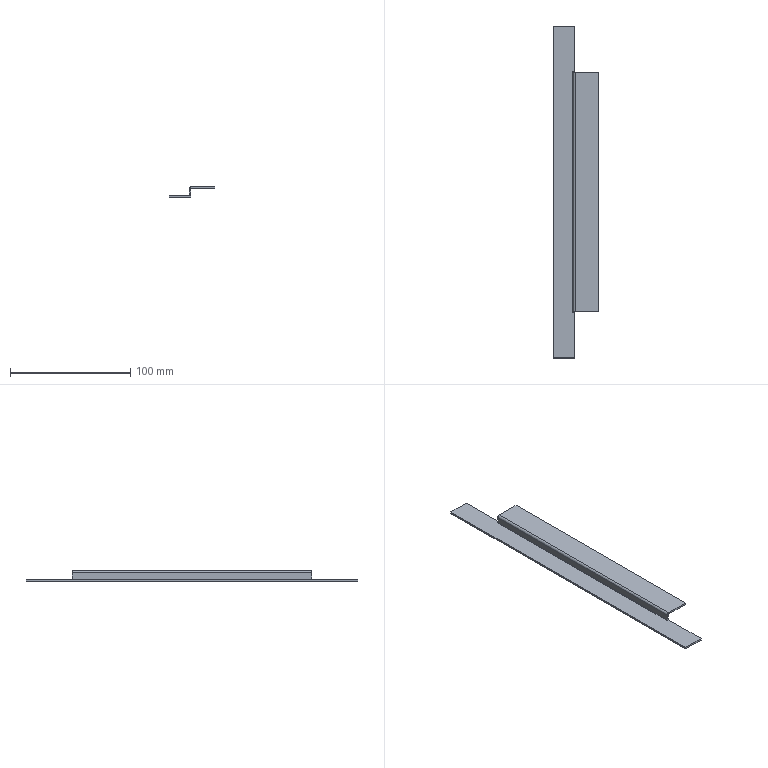Part | SolidWorks | features EdgeFlange 2, FlatPattern 1, SMBaseFlange 1, SheetMetal 1 | 1 solid | 30 faces | box 38.3 x 276.6 x 8.5 mm | volume 15431 mm3 | plane 26 | cylinder 4 | commonest cylinder face diameters 0.4 x2 3.4 x2
STEP:
#1=CARTESIAN_POINT('',(18.3,38.5,0.2));
#2=VERTEX_POINT('',#1);
#3=CARTESIAN_POINT('',(18.3,38.5,5.3));
#4=VERTEX_POINT('',#3);
#5=CARTESIAN_POINT('',(18.3,38.5,7.));
#6=DIRECTION('',(0.,0.,1.));
#7=VECTOR('',#6,1000.);
#8=LINE('',#5,#7);
#9=EDGE_CURVE('',#2,#4,#8,.T.);
#10=ORIENTED_EDGE('',*,*,#9,.T.);
#11=CARTESIAN_POINT('',(16.8,38.5,5.3));
#12=VERTEX_POINT('',#11);
#13=CARTESIAN_POINT('',(18.3,38.5,5.3));
#14=DIRECTION('',(-1.,0.,0.));
#15=VECTOR('',#14,1000.);
#16=LINE('',#13,#15);
#17=EDGE_CURVE('',#4,#12,#16,.T.);
#18=ORIENTED_EDGE('',*,*,#17,.T.);
#19=CARTESIAN_POINT('',(16.8,38.5,0.2));
#20=VERTEX_POINT('',#19);
#21=CARTESIAN_POINT('',(16.8,38.5,0.));
#22=DIRECTION('',(0.,0.,1.));
#23=VECTOR('',#22,1000.);
#24=LINE('',#21,#23);
#25=EDGE_CURVE('',#20,#12,#24,.T.);
#26=ORIENTED_EDGE('',*,*,#25,.F.);
#27=CARTESIAN_POINT('',(18.3,38.5,0.2));
#28=DIRECTION('',(1.,0.,0.));
#29=VECTOR('',#28,1000.);
#30=LINE('',#27,#29);
#31=EDGE_CURVE('',#20,#2,#30,.T.);
#32=ORIENTED_EDGE('',*,*,#31,.T.);
#33=EDGE_LOOP('',(#10,#18,#26,#32));
#34=FACE_OUTER_BOUND('',#33,.T.);
#35=CARTESIAN_POINT('',(18.3,38.5,7.));
#36=DIRECTION('',(0.,-1.,0.));
#37=DIRECTION('',(0.,0.,-1.));
#38=AXIS2_PLACEMENT_3D('',#35,#36,#37);
#39=PLANE('',#38);
#40=ADVANCED_FACE('',(#34),#39,.T.);
#41=CARTESIAN_POINT('',(18.3,238.1,5.3));
#42=VERTEX_POINT('',#41);
#43=CARTESIAN_POINT('',(18.3,238.1,0.2));
#44=VERTEX_POINT('',#43);
#45=CARTESIAN_POINT('',(18.3,238.1,0.));
#46=DIRECTION('',(0.,0.,-1.));
#47=VECTOR('',#46,1000.);
#48=LINE('',#45,#47);
#49=EDGE_CURVE('',#42,#44,#48,.T.);
#50=ORIENTED_EDGE('',*,*,#49,.F.);
#51=CARTESIAN_POINT('',(18.3,38.5,5.3));
#52=DIRECTION('',(0.,1.,0.));
#53=VECTOR('',#52,1000.);
#54=LINE('',#51,#53);
#55=EDGE_CURVE('',#4,#42,#54,.T.);
#56=ORIENTED_EDGE('',*,*,#55,.F.);
#57=ORIENTED_EDGE('',*,*,#9,.F.);
#58=CARTESIAN_POINT('',(18.3,0.,0.2));
#59=DIRECTION('',(0.,1.,0.));
#60=VECTOR('',#59,1000.);
#61=LINE('',#58,#60);
#62=EDGE_CURVE('',#2,#44,#61,.T.);
#63=ORIENTED_EDGE('',*,*,#62,.T.);
#64=EDGE_LOOP('',(#50,#56,#57,#63));
#65=FACE_OUTER_BOUND('',#64,.T.);
#66=CARTESIAN_POINT('',(18.3,0.,0.));
#67=DIRECTION('',(1.,0.,0.));
#68=DIRECTION('',(0.,0.,-1.));
#69=AXIS2_PLACEMENT_3D('',#66,#67,#68);
#70=PLANE('',#69);
#71=ADVANCED_FACE('',(#65),#70,.T.);
#72=CARTESIAN_POINT('',(16.8,238.1,5.3));
#73=VERTEX_POINT('',#72);
#74=CARTESIAN_POINT('',(16.8,38.5,5.3));
#75=DIRECTION('',(0.,1.,0.));
#76=VECTOR('',#75,1000.);
#77=LINE('',#74,#76);
#78=EDGE_CURVE('',#12,#73,#77,.T.);
#79=ORIENTED_EDGE('',*,*,#78,.T.);
#80=CARTESIAN_POINT('',(16.8,238.1,0.2));
#81=VERTEX_POINT('',#80);
#82=CARTESIAN_POINT('',(16.8,238.1,0.));
#83=DIRECTION('',(0.,0.,-1.));
#84=VECTOR('',#83,1000.);
#85=LINE('',#82,#84);
#86=EDGE_CURVE('',#73,#81,#85,.T.);
#87=ORIENTED_EDGE('',*,*,#86,.T.);
#88=CARTESIAN_POINT('',(16.8,38.5,0.2));
#89=DIRECTION('',(0.,1.,0.));
#90=VECTOR('',#89,1000.);
#91=LINE('',#88,#90);
#92=EDGE_CURVE('',#20,#81,#91,.T.);
#93=ORIENTED_EDGE('',*,*,#92,.F.);
#94=ORIENTED_EDGE('',*,*,#25,.T.);
#95=EDGE_LOOP('',(#79,#87,#93,#94));
#96=FACE_OUTER_BOUND('',#95,.T.);
#97=CARTESIAN_POINT('',(16.8,0.,0.));
#98=DIRECTION('',(1.,0.,0.));
#99=DIRECTION('',(0.,0.,-1.));
#100=AXIS2_PLACEMENT_3D('',#97,#98,#99);
#101=PLANE('',#100);
#102=ADVANCED_FACE('',(#96),#101,.F.);
#103=CARTESIAN_POINT('',(18.3,238.4,0.));
#104=VERTEX_POINT('',#103);
#105=CARTESIAN_POINT('',(18.3,276.6,0.));
#106=VERTEX_POINT('',#105);
#107=CARTESIAN_POINT('',(18.3,0.,0.));
#108=DIRECTION('',(0.,1.,0.));
#109=VECTOR('',#108,1000.);
#110=LINE('',#107,#109);
#111=EDGE_CURVE('',#104,#106,#110,.T.);
#112=ORIENTED_EDGE('',*,*,#111,.F.);
#113=CARTESIAN_POINT('',(18.3,238.4,-1.5));
#114=VERTEX_POINT('',#113);
#115=CARTESIAN_POINT('',(18.3,238.4,0.));
#116=DIRECTION('',(0.,0.,-1.));
#117=VECTOR('',#116,1000.);
#118=LINE('',#115,#117);
#119=EDGE_CURVE('',#104,#114,#118,.T.);
#120=ORIENTED_EDGE('',*,*,#119,.T.);
#121=CARTESIAN_POINT('',(18.3,276.6,-1.5));
#122=VERTEX_POINT('',#121);
#123=CARTESIAN_POINT('',(18.3,0.,-1.5));
#124=DIRECTION('',(0.,1.,0.));
#125=VECTOR('',#124,1000.);
#126=LINE('',#123,#125);
#127=EDGE_CURVE('',#114,#122,#126,.T.);
#128=ORIENTED_EDGE('',*,*,#127,.T.);
#129=CARTESIAN_POINT('',(18.3,276.6,-1.5));
#130=DIRECTION('',(0.,0.,1.));
#131=VECTOR('',#130,1000.);
#132=LINE('',#129,#131);
#133=EDGE_CURVE('',#122,#106,#132,.T.);
#134=ORIENTED_EDGE('',*,*,#133,.T.);
#135=EDGE_LOOP('',(#112,#120,#128,#134));
#136=FACE_OUTER_BOUND('',#135,.T.);
#137=CARTESIAN_POINT('',(18.3,0.,-1.5));
#138=DIRECTION('',(1.,0.,0.));
#139=DIRECTION('',(0.,0.,-1.));
#140=AXIS2_PLACEMENT_3D('',#137,#138,#139);
#141=PLANE('',#140);
#142=ADVANCED_FACE('',(#136),#141,.T.);
#143=CARTESIAN_POINT('',(18.3,0.,-1.5));
#144=VERTEX_POINT('',#143);
#145=CARTESIAN_POINT('',(18.3,38.2,-1.5));
#146=VERTEX_POINT('',#145);
#147=CARTESIAN_POINT('',(18.3,0.,-1.5));
#148=DIRECTION('',(0.,1.,0.));
#149=VECTOR('',#148,1000.);
#150=LINE('',#147,#149);
#151=EDGE_CURVE('',#144,#146,#150,.T.);
#152=ORIENTED_EDGE('',*,*,#151,.T.);
#153=CARTESIAN_POINT('',(18.3,38.2,0.));
#154=VERTEX_POINT('',#153);
#155=CARTESIAN_POINT('',(18.3,38.2,0.));
#156=DIRECTION('',(0.,0.,-1.));
#157=VECTOR('',#156,1000.);
#158=LINE('',#155,#157);
#159=EDGE_CURVE('',#154,#146,#158,.T.);
#160=ORIENTED_EDGE('',*,*,#159,.F.);
#161=CARTESIAN_POINT('',(18.3,0.,0.));
#162=VERTEX_POINT('',#161);
#163=CARTESIAN_POINT('',(18.3,0.,0.));
#164=DIRECTION('',(0.,1.,0.));
#165=VECTOR('',#164,1000.);
#166=LINE('',#163,#165);
#167=EDGE_CURVE('',#162,#154,#166,.T.);
#168=ORIENTED_EDGE('',*,*,#167,.F.);
#169=CARTESIAN_POINT('',(18.3,0.,-1.5));
#170=DIRECTION('',(0.,0.,1.));
#171=VECTOR('',#170,1000.);
#172=LINE('',#169,#171);
#173=EDGE_CURVE('',#144,#162,#172,.T.);
#174=ORIENTED_EDGE('',*,*,#173,.F.);
#175=EDGE_LOOP('',(#152,#160,#168,#174));
#176=FACE_OUTER_BOUND('',#175,.T.);
#177=CARTESIAN_POINT('',(18.3,0.,-1.5));
#178=DIRECTION('',(1.,0.,0.));
#179=DIRECTION('',(0.,0.,-1.));
#180=AXIS2_PLACEMENT_3D('',#177,#178,#179);
#181=PLANE('',#180);
#182=ADVANCED_FACE('',(#176),#181,.T.);
#183=ORIENTED_EDGE('',*,*,#127,.F.);
#184=CARTESIAN_POINT('',(16.3,238.4,-1.5));
#185=VERTEX_POINT('',#184);
#186=CARTESIAN_POINT('',(0.,238.4,-1.5));
#187=DIRECTION('',(-1.,0.,0.));
#188=VECTOR('',#187,1000.);
#189=LINE('',#186,#188);
#190=EDGE_CURVE('',#114,#185,#189,.T.);
#191=ORIENTED_EDGE('',*,*,#190,.T.);
#192=CARTESIAN_POINT('',(16.3,238.1,-1.5));
#193=VERTEX_POINT('',#192);
#194=CARTESIAN_POINT('',(16.3,0.,-1.5));
#195=DIRECTION('',(0.,-1.,0.));
#196=VECTOR('',#195,1000.);
#197=LINE('',#194,#196);
#198=EDGE_CURVE('',#185,#193,#197,.T.);
#199=ORIENTED_EDGE('',*,*,#198,.T.);
#200=CARTESIAN_POINT('',(16.6,238.1,-1.5));
#201=VERTEX_POINT('',#200);
#202=CARTESIAN_POINT('',(0.,238.1,-1.5));
#203=DIRECTION('',(1.,0.,0.));
#204=VECTOR('',#203,1000.);
#205=LINE('',#202,#204);
#206=EDGE_CURVE('',#193,#201,#205,.T.);
#207=ORIENTED_EDGE('',*,*,#206,.T.);
#208=CARTESIAN_POINT('',(16.6,38.5,-1.5));
#209=VERTEX_POINT('',#208);
#210=CARTESIAN_POINT('',(16.6,238.1,-1.5));
#211=DIRECTION('',(0.,-1.,0.));
#212=VECTOR('',#211,1000.);
#213=LINE('',#210,#212);
#214=EDGE_CURVE('',#201,#209,#213,.T.);
#215=ORIENTED_EDGE('',*,*,#214,.T.);
#216=CARTESIAN_POINT('',(16.3,38.5,-1.5));
#217=VERTEX_POINT('',#216);
#218=CARTESIAN_POINT('',(0.,38.5,-1.5));
#219=DIRECTION('',(-1.,0.,0.));
#220=VECTOR('',#219,1000.);
#221=LINE('',#218,#220);
#222=EDGE_CURVE('',#209,#217,#221,.T.);
#223=ORIENTED_EDGE('',*,*,#222,.T.);
#224=CARTESIAN_POINT('',(16.3,38.2,-1.5));
#225=VERTEX_POINT('',#224);
#226=CARTESIAN_POINT('',(16.3,0.,-1.5));
#227=DIRECTION('',(0.,-1.,0.));
#228=VECTOR('',#227,1000.);
#229=LINE('',#226,#228);
#230=EDGE_CURVE('',#217,#225,#229,.T.);
#231=ORIENTED_EDGE('',*,*,#230,.T.);
#232=CARTESIAN_POINT('',(0.,38.2,-1.5));
#233=DIRECTION('',(1.,0.,0.));
#234=VECTOR('',#233,1000.);
#235=LINE('',#232,#234);
#236=EDGE_CURVE('',#225,#146,#235,.T.);
#237=ORIENTED_EDGE('',*,*,#236,.T.);
#238=ORIENTED_EDGE('',*,*,#151,.F.);
#239=CARTESIAN_POINT('',(0.,0.,-1.5));
#240=VERTEX_POINT('',#239);
#241=CARTESIAN_POINT('',(0.,0.,-1.5));
#242=DIRECTION('',(1.,0.,0.));
#243=VECTOR('',#242,1000.);
#244=LINE('',#241,#243);
#245=EDGE_CURVE('',#240,#144,#244,.T.);
#246=ORIENTED_EDGE('',*,*,#245,.F.);
#247=CARTESIAN_POINT('',(0.,276.6,-1.5));
#248=VERTEX_POINT('',#247);
#249=CARTESIAN_POINT('',(0.,0.,-1.5));
#250=DIRECTION('',(0.,-1.,0.));
#251=VECTOR('',#250,1000.);
#252=LINE('',#249,#251);
#253=EDGE_CURVE('',#248,#240,#252,.T.);
#254=ORIENTED_EDGE('',*,*,#253,.F.);
#255=CARTESIAN_POINT('',(0.,276.6,-1.5));
#256=DIRECTION('',(-1.,0.,0.));
#257=VECTOR('',#256,1000.);
#258=LINE('',#255,#257);
#259=EDGE_CURVE('',#122,#248,#258,.T.);
#260=ORIENTED_EDGE('',*,*,#259,.F.);
#261=EDGE_LOOP('',(#183,#191,#199,#207,#215,#223,#231,#237,#238,#246,#254,#260));
#262=FACE_OUTER_BOUND('',#261,.T.);
#263=CARTESIAN_POINT('',(0.,0.,-1.5));
#264=DIRECTION('',(0.,0.,-1.));
#265=DIRECTION('',(-1.,0.,0.));
#266=AXIS2_PLACEMENT_3D('',#263,#264,#265);
#267=PLANE('',#266);
#268=ADVANCED_FACE('',(#262),#267,.T.);
#269=CARTESIAN_POINT('',(16.3,238.4,0.));
#270=VERTEX_POINT('',#269);
#271=CARTESIAN_POINT('',(18.3,238.4,0.));
#272=DIRECTION('',(-1.,0.,0.));
#273=VECTOR('',#272,1000.);
#274=LINE('',#271,#273);
#275=EDGE_CURVE('',#104,#270,#274,.T.);
#276=ORIENTED_EDGE('',*,*,#275,.F.);
#277=ORIENTED_EDGE('',*,*,#111,.T.);
#278=CARTESIAN_POINT('',(0.,276.6,0.));
#279=VERTEX_POINT('',#278);
#280=CARTESIAN_POINT('',(0.,276.6,0.));
#281=DIRECTION('',(-1.,0.,0.));
#282=VECTOR('',#281,1000.);
#283=LINE('',#280,#282);
#284=EDGE_CURVE('',#106,#279,#283,.T.);
#285=ORIENTED_EDGE('',*,*,#284,.T.);
#286=CARTESIAN_POINT('',(0.,0.,0.));
#287=VERTEX_POINT('',#286);
#288=CARTESIAN_POINT('',(0.,0.,0.));
#289=DIRECTION('',(0.,-1.,0.));
#290=VECTOR('',#289,1000.);
#291=LINE('',#288,#290);
#292=EDGE_CURVE('',#279,#287,#291,.T.);
#293=ORIENTED_EDGE('',*,*,#292,.T.);
#294=CARTESIAN_POINT('',(0.,0.,0.));
#295=DIRECTION('',(1.,0.,0.));
#296=VECTOR('',#295,1000.);
#297=LINE('',#294,#296);
#298=EDGE_CURVE('',#287,#162,#297,.T.);
#299=ORIENTED_EDGE('',*,*,#298,.T.);
#300=ORIENTED_EDGE('',*,*,#167,.T.);
#301=CARTESIAN_POINT('',(16.3,38.2,0.));
#302=VERTEX_POINT('',#301);
#303=CARTESIAN_POINT('',(16.3,38.2,0.));
#304=DIRECTION('',(1.,0.,0.));
#305=VECTOR('',#304,1000.);
#306=LINE('',#303,#305);
#307=EDGE_CURVE('',#302,#154,#306,.T.);
#308=ORIENTED_EDGE('',*,*,#307,.F.);
#309=CARTESIAN_POINT('',(16.3,38.5,0.));
#310=VERTEX_POINT('',#309);
#311=CARTESIAN_POINT('',(16.3,38.5,0.));
#312=DIRECTION('',(0.,-1.,0.));
#313=VECTOR('',#312,1000.);
#314=LINE('',#311,#313);
#315=EDGE_CURVE('',#310,#302,#314,.T.);
#316=ORIENTED_EDGE('',*,*,#315,.F.);
#317=CARTESIAN_POINT('',(16.6,38.5,0.));
#318=VERTEX_POINT('',#317);
#319=CARTESIAN_POINT('',(16.6,38.5,0.));
#320=DIRECTION('',(-1.,0.,0.));
#321=VECTOR('',#320,1000.);
#322=LINE('',#319,#321);
#323=EDGE_CURVE('',#318,#310,#322,.T.);
#324=ORIENTED_EDGE('',*,*,#323,.F.);
#325=CARTESIAN_POINT('',(16.6,238.1,0.));
#326=VERTEX_POINT('',#325);
#327=CARTESIAN_POINT('',(16.6,238.1,0.));
#328=DIRECTION('',(0.,-1.,0.));
#329=VECTOR('',#328,1000.);
#330=LINE('',#327,#329);
#331=EDGE_CURVE('',#326,#318,#330,.T.);
#332=ORIENTED_EDGE('',*,*,#331,.F.);
#333=CARTESIAN_POINT('',(16.3,238.1,0.));
#334=VERTEX_POINT('',#333);
#335=CARTESIAN_POINT('',(16.3,238.1,0.));
#336=DIRECTION('',(1.,0.,0.));
#337=VECTOR('',#336,1000.);
#338=LINE('',#335,#337);
#339=EDGE_CURVE('',#334,#326,#338,.T.);
#340=ORIENTED_EDGE('',*,*,#339,.F.);
#341=CARTESIAN_POINT('',(16.3,238.4,0.));
#342=DIRECTION('',(0.,-1.,0.));
#343=VECTOR('',#342,1000.);
#344=LINE('',#341,#343);
#345=EDGE_CURVE('',#270,#334,#344,.T.);
#346=ORIENTED_EDGE('',*,*,#345,.F.);
#347=EDGE_LOOP('',(#276,#277,#285,#293,#299,#300,#308,#316,#324,#332,#340,#346));
#348=FACE_OUTER_BOUND('',#347,.T.);
#349=CARTESIAN_POINT('',(0.,0.,0.));
#350=DIRECTION('',(0.,0.,-1.));
#351=DIRECTION('',(-1.,0.,0.));
#352=AXIS2_PLACEMENT_3D('',#349,#350,#351);
#353=PLANE('',#352);
#354=ADVANCED_FACE('',(#348),#353,.F.);
#355=ORIENTED_EDGE('',*,*,#292,.F.);
#356=CARTESIAN_POINT('',(0.,276.6,-1.5));
#357=DIRECTION('',(0.,0.,1.));
#358=VECTOR('',#357,1000.);
#359=LINE('',#356,#358);
#360=EDGE_CURVE('',#248,#279,#359,.T.);
#361=ORIENTED_EDGE('',*,*,#360,.F.);
#362=ORIENTED_EDGE('',*,*,#253,.T.);
#363=CARTESIAN_POINT('',(0.,0.,-1.5));
#364=DIRECTION('',(0.,0.,1.));
#365=VECTOR('',#364,1000.);
#366=LINE('',#363,#365);
#367=EDGE_CURVE('',#240,#287,#366,.T.);
#368=ORIENTED_EDGE('',*,*,#367,.T.);
#369=EDGE_LOOP('',(#355,#361,#362,#368));
#370=FACE_OUTER_BOUND('',#369,.T.);
#371=CARTESIAN_POINT('',(0.,0.,-1.5));
#372=DIRECTION('',(-1.,0.,0.));
#373=DIRECTION('',(0.,0.,1.));
#374=AXIS2_PLACEMENT_3D('',#371,#372,#373);
#375=PLANE('',#374);
#376=ADVANCED_FACE('',(#370),#375,.T.);
#377=ORIENTED_EDGE('',*,*,#284,.F.);
#378=ORIENTED_EDGE('',*,*,#133,.F.);
#379=ORIENTED_EDGE('',*,*,#259,.T.);
#380=ORIENTED_EDGE('',*,*,#360,.T.);
#381=EDGE_LOOP('',(#377,#378,#379,#380));
#382=FACE_OUTER_BOUND('',#381,.T.);
#383=CARTESIAN_POINT('',(0.,276.6,-1.5));
#384=DIRECTION('',(0.,1.,0.));
#385=DIRECTION('',(0.,0.,1.));
#386=AXIS2_PLACEMENT_3D('',#383,#384,#385);
#387=PLANE('',#386);
#388=ADVANCED_FACE('',(#382),#387,.T.);
#389=ORIENTED_EDGE('',*,*,#298,.F.);
#390=ORIENTED_EDGE('',*,*,#367,.F.);
#391=ORIENTED_EDGE('',*,*,#245,.T.);
#392=ORIENTED_EDGE('',*,*,#173,.T.);
#393=EDGE_LOOP('',(#389,#390,#391,#392));
#394=FACE_OUTER_BOUND('',#393,.T.);
#395=CARTESIAN_POINT('',(0.,0.,-1.5));
#396=DIRECTION('',(0.,-1.,0.));
#397=DIRECTION('',(0.,0.,-1.));
#398=AXIS2_PLACEMENT_3D('',#395,#396,#397);
#399=PLANE('',#398);
#400=ADVANCED_FACE('',(#394),#399,.T.);
#401=ORIENTED_EDGE('',*,*,#190,.F.);
#402=ORIENTED_EDGE('',*,*,#119,.F.);
#403=ORIENTED_EDGE('',*,*,#275,.T.);
#404=CARTESIAN_POINT('',(16.3,238.4,0.));
#405=DIRECTION('',(0.,0.,-1.));
#406=VECTOR('',#405,1000.);
#407=LINE('',#404,#406);
#408=EDGE_CURVE('',#270,#185,#407,.T.);
#409=ORIENTED_EDGE('',*,*,#408,.T.);
#410=EDGE_LOOP('',(#401,#402,#403,#409));
#411=FACE_OUTER_BOUND('',#410,.T.);
#412=CARTESIAN_POINT('',(18.3,238.4,0.));
#413=DIRECTION('',(0.,-1.,0.));
#414=DIRECTION('',(0.,0.,-1.));
#415=AXIS2_PLACEMENT_3D('',#412,#413,#414);
#416=PLANE('',#415);
#417=ADVANCED_FACE('',(#411),#416,.T.);
#418=ORIENTED_EDGE('',*,*,#198,.F.);
#419=ORIENTED_EDGE('',*,*,#408,.F.);
#420=ORIENTED_EDGE('',*,*,#345,.T.);
#421=CARTESIAN_POINT('',(16.3,238.1,0.));
#422=DIRECTION('',(0.,0.,-1.));
#423=VECTOR('',#422,1000.);
#424=LINE('',#421,#423);
#425=EDGE_CURVE('',#334,#193,#424,.T.);
#426=ORIENTED_EDGE('',*,*,#425,.T.);
#427=EDGE_LOOP('',(#418,#419,#420,#426));
#428=FACE_OUTER_BOUND('',#427,.T.);
#429=CARTESIAN_POINT('',(16.3,238.4,0.));
#430=DIRECTION('',(1.,0.,0.));
#431=DIRECTION('',(0.,0.,-1.));
#432=AXIS2_PLACEMENT_3D('',#429,#430,#431);
#433=PLANE('',#432);
#434=ADVANCED_FACE('',(#428),#433,.T.);
#435=ORIENTED_EDGE('',*,*,#206,.F.);
#436=ORIENTED_EDGE('',*,*,#425,.F.);
#437=ORIENTED_EDGE('',*,*,#339,.T.);
#438=CARTESIAN_POINT('',(16.6,238.1,0.));
#439=DIRECTION('',(0.,0.,-1.));
#440=VECTOR('',#439,1000.);
#441=LINE('',#438,#440);
#442=EDGE_CURVE('',#326,#201,#441,.T.);
#443=ORIENTED_EDGE('',*,*,#442,.T.);
#444=EDGE_LOOP('',(#435,#436,#437,#443));
#445=FACE_OUTER_BOUND('',#444,.T.);
#446=CARTESIAN_POINT('',(16.3,238.1,0.));
#447=DIRECTION('',(0.,1.,0.));
#448=DIRECTION('',(0.,0.,1.));
#449=AXIS2_PLACEMENT_3D('',#446,#447,#448);
#450=PLANE('',#449);
#451=ADVANCED_FACE('',(#445),#450,.T.);
#452=ORIENTED_EDGE('',*,*,#222,.F.);
#453=CARTESIAN_POINT('',(16.6,38.5,0.));
#454=DIRECTION('',(0.,0.,-1.));
#455=VECTOR('',#454,1000.);
#456=LINE('',#453,#455);
#457=EDGE_CURVE('',#318,#209,#456,.T.);
#458=ORIENTED_EDGE('',*,*,#457,.F.);
#459=ORIENTED_EDGE('',*,*,#323,.T.);
#460=CARTESIAN_POINT('',(16.3,38.5,0.));
#461=DIRECTION('',(0.,0.,-1.));
#462=VECTOR('',#461,1000.);
#463=LINE('',#460,#462);
#464=EDGE_CURVE('',#310,#217,#463,.T.);
#465=ORIENTED_EDGE('',*,*,#464,.T.);
#466=EDGE_LOOP('',(#452,#458,#459,#465));
#467=FACE_OUTER_BOUND('',#466,.T.);
#468=CARTESIAN_POINT('',(16.6,38.5,0.));
#469=DIRECTION('',(0.,-1.,0.));
#470=DIRECTION('',(0.,0.,-1.));
#471=AXIS2_PLACEMENT_3D('',#468,#469,#470);
#472=PLANE('',#471);
#473=ADVANCED_FACE('',(#467),#472,.T.);
#474=ORIENTED_EDGE('',*,*,#230,.F.);
#475=ORIENTED_EDGE('',*,*,#464,.F.);
#476=ORIENTED_EDGE('',*,*,#315,.T.);
#477=CARTESIAN_POINT('',(16.3,38.2,0.));
#478=DIRECTION('',(0.,0.,-1.));
#479=VECTOR('',#478,1000.);
#480=LINE('',#477,#479);
#481=EDGE_CURVE('',#302,#225,#480,.T.);
#482=ORIENTED_EDGE('',*,*,#481,.T.);
#483=EDGE_LOOP('',(#474,#475,#476,#482));
#484=FACE_OUTER_BOUND('',#483,.T.);
#485=CARTESIAN_POINT('',(16.3,38.5,0.));
#486=DIRECTION('',(1.,0.,0.));
#487=DIRECTION('',(0.,0.,-1.));
#488=AXIS2_PLACEMENT_3D('',#485,#486,#487);
#489=PLANE('',#488);
#490=ADVANCED_FACE('',(#484),#489,.T.);
#491=ORIENTED_EDGE('',*,*,#236,.F.);
#492=ORIENTED_EDGE('',*,*,#481,.F.);
#493=ORIENTED_EDGE('',*,*,#307,.T.);
#494=ORIENTED_EDGE('',*,*,#159,.T.);
#495=EDGE_LOOP('',(#491,#492,#493,#494));
#496=FACE_OUTER_BOUND('',#495,.T.);
#497=CARTESIAN_POINT('',(16.3,38.2,0.));
#498=DIRECTION('',(0.,1.,0.));
#499=DIRECTION('',(0.,0.,1.));
#500=AXIS2_PLACEMENT_3D('',#497,#498,#499);
#501=PLANE('',#500);
#502=ADVANCED_FACE('',(#496),#501,.T.);
#503=ORIENTED_EDGE('',*,*,#31,.F.);
#504=CARTESIAN_POINT('',(16.6,38.5,0.2));
#505=DIRECTION('',(0.,-1.,0.));
#506=DIRECTION('',(0.,0.,1.));
#507=AXIS2_PLACEMENT_3D('',#504,#505,#506);
#508=CIRCLE('',#507,0.2);
#509=EDGE_CURVE('',#318,#20,#508,.T.);
#510=ORIENTED_EDGE('',*,*,#509,.F.);
#511=ORIENTED_EDGE('',*,*,#457,.T.);
#512=CARTESIAN_POINT('',(16.6,38.5,0.2));
#513=DIRECTION('',(0.,-1.,0.));
#514=DIRECTION('',(0.,0.,1.));
#515=AXIS2_PLACEMENT_3D('',#512,#513,#514);
#516=CIRCLE('',#515,1.7);
#517=EDGE_CURVE('',#209,#2,#516,.T.);
#518=ORIENTED_EDGE('',*,*,#517,.T.);
#519=EDGE_LOOP('',(#503,#510,#511,#518));
#520=FACE_OUTER_BOUND('',#519,.T.);
#521=CARTESIAN_POINT('',(16.6,38.5,0.2));
#522=DIRECTION('',(0.,-1.,0.));
#523=DIRECTION('',(0.,0.,-1.));
#524=AXIS2_PLACEMENT_3D('',#521,#522,#523);
#525=PLANE('',#524);
#526=ADVANCED_FACE('',(#520),#525,.T.);
#527=CARTESIAN_POINT('',(16.6,238.1,0.2));
#528=DIRECTION('',(0.,1.,0.));
#529=DIRECTION('',(0.,0.,1.));
#530=AXIS2_PLACEMENT_3D('',#527,#528,#529);
#531=CIRCLE('',#530,0.2);
#532=EDGE_CURVE('',#81,#326,#531,.T.);
#533=ORIENTED_EDGE('',*,*,#532,.F.);
#534=CARTESIAN_POINT('',(16.8,238.1,0.2));
#535=DIRECTION('',(1.,0.,0.));
#536=VECTOR('',#535,1000.);
#537=LINE('',#534,#536);
#538=EDGE_CURVE('',#81,#44,#537,.T.);
#539=ORIENTED_EDGE('',*,*,#538,.T.);
#540=CARTESIAN_POINT('',(16.6,238.1,0.2));
#541=DIRECTION('',(0.,1.,0.));
#542=DIRECTION('',(0.,0.,1.));
#543=AXIS2_PLACEMENT_3D('',#540,#541,#542);
#544=CIRCLE('',#543,1.7);
#545=EDGE_CURVE('',#44,#201,#544,.T.);
#546=ORIENTED_EDGE('',*,*,#545,.T.);
#547=ORIENTED_EDGE('',*,*,#442,.F.);
#548=EDGE_LOOP('',(#533,#539,#546,#547));
#549=FACE_OUTER_BOUND('',#548,.T.);
#550=CARTESIAN_POINT('',(16.6,238.1,0.2));
#551=DIRECTION('',(0.,-1.,0.));
#552=DIRECTION('',(0.,0.,-1.));
#553=AXIS2_PLACEMENT_3D('',#550,#551,#552);
#554=PLANE('',#553);
#555=ADVANCED_FACE('',(#549),#554,.F.);
#556=ORIENTED_EDGE('',*,*,#214,.F.);
#557=ORIENTED_EDGE('',*,*,#545,.F.);
#558=ORIENTED_EDGE('',*,*,#62,.F.);
#559=ORIENTED_EDGE('',*,*,#517,.F.);
#560=EDGE_LOOP('',(#556,#557,#558,#559));
#561=FACE_OUTER_BOUND('',#560,.T.);
#562=CARTESIAN_POINT('',(16.6,238.1,0.2));
#563=DIRECTION('',(0.,1.,0.));
#564=DIRECTION('',(1.,0.,0.));
#565=AXIS2_PLACEMENT_3D('',#562,#563,#564);
#566=CYLINDRICAL_SURFACE('',#565,1.7);
#567=ADVANCED_FACE('',(#561),#566,.T.);
#568=ORIENTED_EDGE('',*,*,#331,.T.);
#569=ORIENTED_EDGE('',*,*,#509,.T.);
#570=ORIENTED_EDGE('',*,*,#92,.T.);
#571=ORIENTED_EDGE('',*,*,#532,.T.);
#572=EDGE_LOOP('',(#568,#569,#570,#571));
#573=FACE_OUTER_BOUND('',#572,.T.);
#574=CARTESIAN_POINT('',(16.6,238.1,0.2));
#575=DIRECTION('',(0.,1.,0.));
#576=DIRECTION('',(1.,0.,0.));
#577=AXIS2_PLACEMENT_3D('',#574,#575,#576);
#578=CYLINDRICAL_SURFACE('',#577,0.2);
#579=ADVANCED_FACE('',(#573),#578,.F.);
#580=CARTESIAN_POINT('',(18.3,238.1,5.3));
#581=DIRECTION('',(-1.,0.,0.));
#582=VECTOR('',#581,1000.);
#583=LINE('',#580,#582);
#584=EDGE_CURVE('',#42,#73,#583,.T.);
#585=ORIENTED_EDGE('',*,*,#584,.F.);
#586=ORIENTED_EDGE('',*,*,#49,.T.);
#587=ORIENTED_EDGE('',*,*,#538,.F.);
#588=ORIENTED_EDGE('',*,*,#86,.F.);
#589=EDGE_LOOP('',(#585,#586,#587,#588));
#590=FACE_OUTER_BOUND('',#589,.T.);
#591=CARTESIAN_POINT('',(18.3,238.1,0.));
#592=DIRECTION('',(0.,1.,0.));
#593=DIRECTION('',(0.,0.,1.));
#594=AXIS2_PLACEMENT_3D('',#591,#592,#593);
#595=PLANE('',#594);
#596=ADVANCED_FACE('',(#590),#595,.T.);
#597=CARTESIAN_POINT('',(18.5,238.1,5.5));
#598=VERTEX_POINT('',#597);
#599=CARTESIAN_POINT('',(18.5,238.1,7.));
#600=VERTEX_POINT('',#599);
#601=CARTESIAN_POINT('',(18.5,238.1,7.));
#602=DIRECTION('',(0.,0.,1.));
#603=VECTOR('',#602,1000.);
#604=LINE('',#601,#603);
#605=EDGE_CURVE('',#598,#600,#604,.T.);
#606=ORIENTED_EDGE('',*,*,#605,.F.);
#607=CARTESIAN_POINT('',(18.5,238.1,5.3));
#608=DIRECTION('',(0.,1.,0.));
#609=DIRECTION('',(0.,0.,-1.));
#610=AXIS2_PLACEMENT_3D('',#607,#608,#609);
#611=CIRCLE('',#610,0.2);
#612=EDGE_CURVE('',#42,#598,#611,.T.);
#613=ORIENTED_EDGE('',*,*,#612,.F.);
#614=ORIENTED_EDGE('',*,*,#584,.T.);
#615=CARTESIAN_POINT('',(18.5,238.1,5.3));
#616=DIRECTION('',(0.,1.,0.));
#617=DIRECTION('',(0.,0.,-1.));
#618=AXIS2_PLACEMENT_3D('',#615,#616,#617);
#619=CIRCLE('',#618,1.7);
#620=EDGE_CURVE('',#73,#600,#619,.T.);
#621=ORIENTED_EDGE('',*,*,#620,.T.);
#622=EDGE_LOOP('',(#606,#613,#614,#621));
#623=FACE_OUTER_BOUND('',#622,.T.);
#624=CARTESIAN_POINT('',(18.5,238.1,5.3));
#625=DIRECTION('',(0.,1.,0.));
#626=DIRECTION('',(0.,0.,1.));
#627=AXIS2_PLACEMENT_3D('',#624,#625,#626);
#628=PLANE('',#627);
#629=ADVANCED_FACE('',(#623),#628,.T.);
#630=CARTESIAN_POINT('',(18.5,38.5,5.5));
#631=VERTEX_POINT('',#630);
#632=CARTESIAN_POINT('',(18.5,38.5,5.3));
#633=DIRECTION('',(0.,-1.,0.));
#634=DIRECTION('',(0.,0.,-1.));
#635=AXIS2_PLACEMENT_3D('',#632,#633,#634);
#636=CIRCLE('',#635,0.2);
#637=EDGE_CURVE('',#631,#4,#636,.T.);
#638=ORIENTED_EDGE('',*,*,#637,.F.);
#639=CARTESIAN_POINT('',(18.5,38.5,7.));
#640=VERTEX_POINT('',#639);
#641=CARTESIAN_POINT('',(18.5,38.5,5.5));
#642=DIRECTION('',(0.,0.,1.));
#643=VECTOR('',#642,1000.);
#644=LINE('',#641,#643);
#645=EDGE_CURVE('',#631,#640,#644,.T.);
#646=ORIENTED_EDGE('',*,*,#645,.T.);
#647=CARTESIAN_POINT('',(18.5,38.5,5.3));
#648=DIRECTION('',(0.,-1.,0.));
#649=DIRECTION('',(0.,0.,-1.));
#650=AXIS2_PLACEMENT_3D('',#647,#648,#649);
#651=CIRCLE('',#650,1.7);
#652=EDGE_CURVE('',#640,#12,#651,.T.);
#653=ORIENTED_EDGE('',*,*,#652,.T.);
#654=ORIENTED_EDGE('',*,*,#17,.F.);
#655=EDGE_LOOP('',(#638,#646,#653,#654));
#656=FACE_OUTER_BOUND('',#655,.T.);
#657=CARTESIAN_POINT('',(18.5,38.5,5.3));
#658=DIRECTION('',(0.,1.,0.));
#659=DIRECTION('',(0.,0.,1.));
#660=AXIS2_PLACEMENT_3D('',#657,#658,#659);
#661=PLANE('',#660);
#662=ADVANCED_FACE('',(#656),#661,.F.);
#663=ORIENTED_EDGE('',*,*,#78,.F.);
#664=ORIENTED_EDGE('',*,*,#652,.F.);
#665=CARTESIAN_POINT('',(18.5,0.,7.));
#666=DIRECTION('',(0.,-1.,0.));
#667=VECTOR('',#666,1000.);
#668=LINE('',#665,#667);
#669=EDGE_CURVE('',#600,#640,#668,.T.);
#670=ORIENTED_EDGE('',*,*,#669,.F.);
#671=ORIENTED_EDGE('',*,*,#620,.F.);
#672=EDGE_LOOP('',(#663,#664,#670,#671));
#673=FACE_OUTER_BOUND('',#672,.T.);
#674=CARTESIAN_POINT('',(18.5,38.5,5.3));
#675=DIRECTION('',(0.,-1.,0.));
#676=DIRECTION('',(0.,0.,1.));
#677=AXIS2_PLACEMENT_3D('',#674,#675,#676);
#678=CYLINDRICAL_SURFACE('',#677,1.7);
#679=ADVANCED_FACE('',(#673),#678,.T.);
#680=ORIENTED_EDGE('',*,*,#55,.T.);
#681=ORIENTED_EDGE('',*,*,#612,.T.);
#682=CARTESIAN_POINT('',(18.5,238.1,5.5));
#683=DIRECTION('',(0.,-1.,0.));
#684=VECTOR('',#683,1000.);
#685=LINE('',#682,#684);
#686=EDGE_CURVE('',#598,#631,#685,.T.);
#687=ORIENTED_EDGE('',*,*,#686,.T.);
#688=ORIENTED_EDGE('',*,*,#637,.T.);
#689=EDGE_LOOP('',(#680,#681,#687,#688));
#690=FACE_OUTER_BOUND('',#689,.T.);
#691=CARTESIAN_POINT('',(18.5,38.5,5.3));
#692=DIRECTION('',(0.,-1.,0.));
#693=DIRECTION('',(0.,0.,1.));
#694=AXIS2_PLACEMENT_3D('',#691,#692,#693);
#695=CYLINDRICAL_SURFACE('',#694,0.2);
#696=ADVANCED_FACE('',(#690),#695,.F.);
#697=CARTESIAN_POINT('',(38.3,38.5,7.));
#698=VERTEX_POINT('',#697);
#699=CARTESIAN_POINT('',(18.3,38.5,7.));
#700=DIRECTION('',(-1.,0.,0.));
#701=VECTOR('',#700,1000.);
#702=LINE('',#699,#701);
#703=EDGE_CURVE('',#698,#640,#702,.T.);
#704=ORIENTED_EDGE('',*,*,#703,.T.);
#705=ORIENTED_EDGE('',*,*,#645,.F.);
#706=CARTESIAN_POINT('',(38.3,38.5,5.5));
#707=VERTEX_POINT('',#706);
#708=CARTESIAN_POINT('',(0.,38.5,5.5));
#709=DIRECTION('',(-1.,0.,0.));
#710=VECTOR('',#709,1000.);
#711=LINE('',#708,#710);
#712=EDGE_CURVE('',#707,#631,#711,.T.);
#713=ORIENTED_EDGE('',*,*,#712,.F.);
#714=CARTESIAN_POINT('',(38.3,38.5,7.));
#715=DIRECTION('',(0.,0.,-1.));
#716=VECTOR('',#715,1000.);
#717=LINE('',#714,#716);
#718=EDGE_CURVE('',#698,#707,#717,.T.);
#719=ORIENTED_EDGE('',*,*,#718,.F.);
#720=EDGE_LOOP('',(#704,#705,#713,#719));
#721=FACE_OUTER_BOUND('',#720,.T.);
#722=CARTESIAN_POINT('',(18.3,38.5,7.));
#723=DIRECTION('',(0.,-1.,0.));
#724=DIRECTION('',(0.,0.,-1.));
#725=AXIS2_PLACEMENT_3D('',#722,#723,#724);
#726=PLANE('',#725);
#727=ADVANCED_FACE('',(#721),#726,.T.);
#728=CARTESIAN_POINT('',(38.3,238.1,5.5));
#729=VERTEX_POINT('',#728);
#730=CARTESIAN_POINT('',(0.,238.1,5.5));
#731=DIRECTION('',(1.,0.,0.));
#732=VECTOR('',#731,1000.);
#733=LINE('',#730,#732);
#734=EDGE_CURVE('',#598,#729,#733,.T.);
#735=ORIENTED_EDGE('',*,*,#734,.F.);
#736=ORIENTED_EDGE('',*,*,#605,.T.);
#737=CARTESIAN_POINT('',(38.3,238.1,7.));
#738=VERTEX_POINT('',#737);
#739=CARTESIAN_POINT('',(38.3,238.1,7.));
#740=DIRECTION('',(1.,0.,0.));
#741=VECTOR('',#740,1000.);
#742=LINE('',#739,#741);
#743=EDGE_CURVE('',#600,#738,#742,.T.);
#744=ORIENTED_EDGE('',*,*,#743,.T.);
#745=CARTESIAN_POINT('',(38.3,238.1,7.));
#746=DIRECTION('',(0.,0.,-1.));
#747=VECTOR('',#746,1000.);
#748=LINE('',#745,#747);
#749=EDGE_CURVE('',#738,#729,#748,.T.);
#750=ORIENTED_EDGE('',*,*,#749,.T.);
#751=EDGE_LOOP('',(#735,#736,#744,#750));
#752=FACE_OUTER_BOUND('',#751,.T.);
#753=CARTESIAN_POINT('',(38.3,238.1,7.));
#754=DIRECTION('',(0.,1.,0.));
#755=DIRECTION('',(0.,0.,1.));
#756=AXIS2_PLACEMENT_3D('',#753,#754,#755);
#757=PLANE('',#756);
#758=ADVANCED_FACE('',(#752),#757,.T.);
#759=ORIENTED_EDGE('',*,*,#743,.F.);
#760=ORIENTED_EDGE('',*,*,#669,.T.);
#761=ORIENTED_EDGE('',*,*,#703,.F.);
#762=CARTESIAN_POINT('',(38.3,38.5,7.));
#763=DIRECTION('',(0.,-1.,0.));
#764=VECTOR('',#763,1000.);
#765=LINE('',#762,#764);
#766=EDGE_CURVE('',#738,#698,#765,.T.);
#767=ORIENTED_EDGE('',*,*,#766,.F.);
#768=EDGE_LOOP('',(#759,#760,#761,#767));
#769=FACE_OUTER_BOUND('',#768,.T.);
#770=CARTESIAN_POINT('',(0.,0.,7.));
#771=DIRECTION('',(0.,0.,1.));
#772=DIRECTION('',(1.,0.,0.));
#773=AXIS2_PLACEMENT_3D('',#770,#771,#772);
#774=PLANE('',#773);
#775=ADVANCED_FACE('',(#769),#774,.T.);
#776=ORIENTED_EDGE('',*,*,#686,.F.);
#777=ORIENTED_EDGE('',*,*,#734,.T.);
#778=CARTESIAN_POINT('',(38.3,0.,5.5));
#779=DIRECTION('',(0.,-1.,0.));
#780=VECTOR('',#779,1000.);
#781=LINE('',#778,#780);
#782=EDGE_CURVE('',#729,#707,#781,.T.);
#783=ORIENTED_EDGE('',*,*,#782,.T.);
#784=ORIENTED_EDGE('',*,*,#712,.T.);
#785=EDGE_LOOP('',(#776,#777,#783,#784));
#786=FACE_OUTER_BOUND('',#785,.T.);
#787=CARTESIAN_POINT('',(0.,0.,5.5));
#788=DIRECTION('',(0.,0.,1.));
#789=DIRECTION('',(1.,0.,0.));
#790=AXIS2_PLACEMENT_3D('',#787,#788,#789);
#791=PLANE('',#790);
#792=ADVANCED_FACE('',(#786),#791,.F.);
#793=ORIENTED_EDGE('',*,*,#782,.F.);
#794=ORIENTED_EDGE('',*,*,#749,.F.);
#795=ORIENTED_EDGE('',*,*,#766,.T.);
#796=ORIENTED_EDGE('',*,*,#718,.T.);
#797=EDGE_LOOP('',(#793,#794,#795,#796));
#798=FACE_OUTER_BOUND('',#797,.T.);
#799=CARTESIAN_POINT('',(38.3,38.5,7.));
#800=DIRECTION('',(1.,0.,0.));
#801=DIRECTION('',(0.,0.,-1.));
#802=AXIS2_PLACEMENT_3D('',#799,#800,#801);
#803=PLANE('',#802);
#804=ADVANCED_FACE('',(#798),#803,.T.);
#805=CLOSED_SHELL('',(#40,#71,#102,#142,#182,#268,#354,#376,#388,#400,#417,#434,#451,#473,#490,#502,#526,#555,#567,#579,#596,#629,#662,#679,#696,#727,#758,#775,#792,#804));
#806=MANIFOLD_SOLID_BREP('',#805);
#807=CARTESIAN_POINT('',(0.,0.,0.));
#808=DIRECTION('',(0.,0.,1.));
#809=DIRECTION('',(1.,0.,0.));
#810=AXIS2_PLACEMENT_3D('',#807,#808,#809);
#811=(LENGTH_UNIT()NAMED_UNIT(*)SI_UNIT(.MILLI.,.METRE.));
#812=UNCERTAINTY_MEASURE_WITH_UNIT(LENGTH_MEASURE(0.00001),#811,'','');
#813=(NAMED_UNIT(*)PLANE_ANGLE_UNIT()SI_UNIT($,.RADIAN.));
#814=(NAMED_UNIT(*)SI_UNIT($,.STERADIAN.)SOLID_ANGLE_UNIT());
#815=(GEOMETRIC_REPRESENTATION_CONTEXT(3)GLOBAL_UNCERTAINTY_ASSIGNED_CONTEXT((#812))GLOBAL_UNIT_ASSIGNED_CONTEXT((#811,#813,#814))REPRESENTATION_CONTEXT('',''));
#816=ADVANCED_BREP_SHAPE_REPRESENTATION('',(#806,#810),#815);